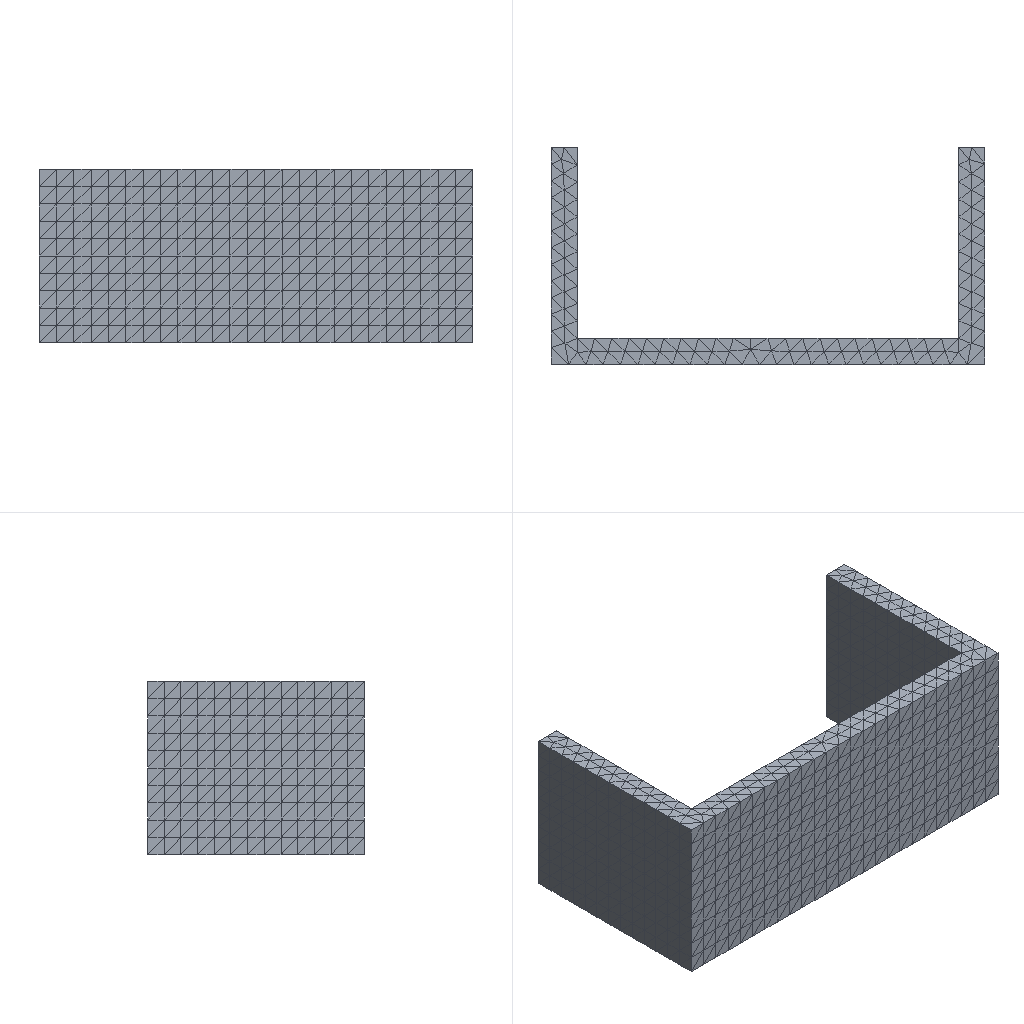Simulation study | abaqus
Notes in the study folder:
11 U clamp
job_status=None
Umax_mm=0.0764947
S_Mises_max_MPa=77.88
Set-up summary:
category,name,step,type,value,unit,region
solver,abaqus,,Abaqus/CAE 2024
units,mm-N-s-tonne (MPa),,inferred,E=210000 density=7.85e-09
analysis,Step-1,,static,time_period=1
mesh,nodes,,,9834
mesh,elements,,,5528
element_type,C3D10,,,5528
material,Steel,,E,210000
material,Steel,,nu,0.3
material,Steel,,density,7.85e-09
section,Steel,,solid section,,,_PickedSet2
load,PL,Step-1,pressure,0.5,,L
load,PR,Step-1,pressure,0.5,,R
bc,BC,Step-1,encastre,[dofs=ENCASTRE],,FIXED
Abaqus input file, long lists of numbers shortened:
*Heading
** Job name: deck Model name: M11
** Generated by: Abaqus/CAE 2024
*Preprint, echo=NO, model=NO, history=NO, contact=NO
**
** PARTS
**
*Part, name=P
*Node
      1,         -44.,          50.,          40.
      2,         -44.,           6.,          40.
** (9832 more lines like these left out)
*Element, type=C3D10
   1, 1184, 1185,  355,  356, 1566, 1565, 1564, 1568, 1567, 1569
   2, 1184, 1185,  868,  869, 1566, 1571, 1570, 1573, 1572, 1574
** (5526 more lines like these left out)
*Nset, nset=_PickedSet2, internal, generate
    1,  9834,     1
*Elset, elset=_PickedSet2, internal, generate
    1,  5528,     1
** Section: Sec
*Solid Section, elset=_PickedSet2, material=Steel
,
*End Part
**
**
** ASSEMBLY
**
*Assembly, name=Assembly
**
*Instance, name=I, part=P
*End Instance
**
*Nset, nset=FIXED, instance=I
    7,    8,    9,   10,  106,  107,  108,  109,  110,  111,  112,  113,  114,  115,  116,  117
  118,  119,  120,  121,  122,  123,  124,  125,  126,  127,  128,  129,  130,  131,  132,  133
** (65 more lines like these left out)
*Elset, elset=FIXED, instance=I
   68,  107,  124,  151,  157,  165,  177,  181,  194,  220,  237,  482,  486,  491,  501,  676
  682,  700,  702,  709,  715,  717,  762,  764,  774,  832,  833,  908,  918,  932,  934,  935
** (30 more lines like these left out)
*Elset, elset=_L_S3, internal, instance=I
   80,  254,  257,  270,  273,  340,  347,  393,  424,  503,  514,  534,  580,  663,  725,  867
  888,  931,  998, 1024, 1238, 1247, 1294, 1307, 1363, 1386, 1451, 1570, 1596, 1599, 1602, 1604
** (10 more lines like these left out)
*Elset, elset=_L_S4, internal, instance=I
  168, 2010, 2063, 2070, 2506, 4124, 5291, 5445
*Elset, elset=_L_S2, internal, instance=I
  269, 1821, 1822, 1939, 1990, 2449, 2491, 3777, 4765, 5146, 5176, 5374
*Elset, elset=_L_S1, internal, instance=I
  569,  865, 1709, 1732, 1736, 1901, 2132, 2293, 2408, 2414, 2508, 3004, 3428, 5186, 5302
*Surface, type=ELEMENT, name=L
_L_S3, S3
_L_S4, S4
_L_S2, S2
_L_S1, S1
*Elset, elset=_R_S3, internal, instance=I
  121,  233,  315,  381,  432,  456,  460,  469,  642,  803,  822, 1259, 1383, 1427, 1460, 1535
 1549, 1647, 1728, 1766, 1796, 1934, 1963, 1983, 2116, 2117, 2261, 2309, 2335, 2352, 2372, 2598
** (11 more lines like these left out)
*Elset, elset=_R_S4, internal, instance=I
 3851, 3862, 4192, 5112, 5117, 5258
*Elset, elset=_R_S1, internal, instance=I
 4189, 4357, 4471, 4544, 5012, 5059, 5130
*Elset, elset=_R_S2, internal, instance=I
 4334, 4530, 5416
*Surface, type=ELEMENT, name=R
_R_S3, S3
_R_S4, S4
_R_S2, S2
_R_S1, S1
*End Assembly
**
** MATERIALS
**
*Material, name=Steel
*Density
 7.85e-09,
*Elastic
210000., 0.3
** ----------------------------------------------------------------
**
** STEP: Step-1
**
*Step, name=Step-1, nlgeom=NO
*Static
1., 1., 1e-05, 1.
**
** BOUNDARY CONDITIONS
**
** Name: BC Type: Symmetry/Antisymmetry/Encastre
*Boundary
FIXED, ENCASTRE
**
** LOADS
**
** Name: PL   Type: Pressure
*Dsload
L, P, 0.5
** Name: PR   Type: Pressure
*Dsload
R, P, 0.5
**
** OUTPUT REQUESTS
**
*Restart, write, frequency=0
**
** FIELD OUTPUT: F-Output-1
**
*Output, field, variable=PRESELECT
**
** HISTORY OUTPUT: H-Output-1
**
*Output, history, variable=PRESELECT
*End Step
Results summary:
result,odb.job_status,,,JOB_STATUS_COMPLETED_SUCCESSFULLY,"consistent, unstated (Abaqus has no unit system)"
result,steps[0].procedure,Step-1,,*STATIC,"consistent, unstated (Abaqus has no unit system)"
result,steps[0].time_period,Step-1,,1,"consistent, unstated (Abaqus has no unit system)"
result,steps[0].n_frames,Step-1,,2,"consistent, unstated (Abaqus has no unit system)"
result,steps[0].last_frame.id,Step-1,,1,"consistent, unstated (Abaqus has no unit system)"
result,steps[0].last_frame.value,Step-1,,1,"consistent, unstated (Abaqus has no unit system)"
result,steps[0].last_frame.description,Step-1,,Increment      1: Step Time =    1.000,"consistent, unstated (Abaqus has no unit system)"
result,steps[0].completed,Step-1,,True,"consistent, unstated (Abaqus has no unit system)"
result,steps[0].max_U_magnitude,Step-1,,0.07649,"consistent, unstated (Abaqus has no unit system)"
result,steps[0].max_S_mises,Step-1,,77.88,"consistent, unstated (Abaqus has no unit system)"
result,steps[0].RF_sum[1],Step-1,,-0.0001087,"consistent, unstated (Abaqus has no unit system)"
result,steps[0].RF_sum[2],Step-1,,-0.0001507,"consistent, unstated (Abaqus has no unit system)"
result,steps[0].RF_sum[3],Step-1,,-1.52588e-05,"consistent, unstated (Abaqus has no unit system)"
result,steps[1].procedure,Step-1,,*STATIC,"consistent, unstated (Abaqus has no unit system)"
result,steps[1].time_period,Step-1,,1,"consistent, unstated (Abaqus has no unit system)"
result,steps[1].n_frames,Step-1,,2,"consistent, unstated (Abaqus has no unit system)"
result,steps[1].last_frame.id,Step-1,,1,"consistent, unstated (Abaqus has no unit system)"
result,steps[1].last_frame.value,Step-1,,1,"consistent, unstated (Abaqus has no unit system)"
result,steps[1].last_frame.description,Step-1,,Increment      1: Step Time =    1.000,"consistent, unstated (Abaqus has no unit system)"
result,steps[1].completed,Step-1,,True,"consistent, unstated (Abaqus has no unit system)"
result,steps[1].max_U_magnitude,Step-1,,0.07649,"consistent, unstated (Abaqus has no unit system)"
result,steps[1].max_S_mises,Step-1,,77.88,"consistent, unstated (Abaqus has no unit system)"
result,steps[1].RF_sum[1],Step-1,,-0.0001087,"consistent, unstated (Abaqus has no unit system)"
result,steps[1].RF_sum[2],Step-1,,-0.0001507,"consistent, unstated (Abaqus has no unit system)"
result,steps[1].RF_sum[3],Step-1,,-1.52588e-05,"consistent, unstated (Abaqus has no unit system)"